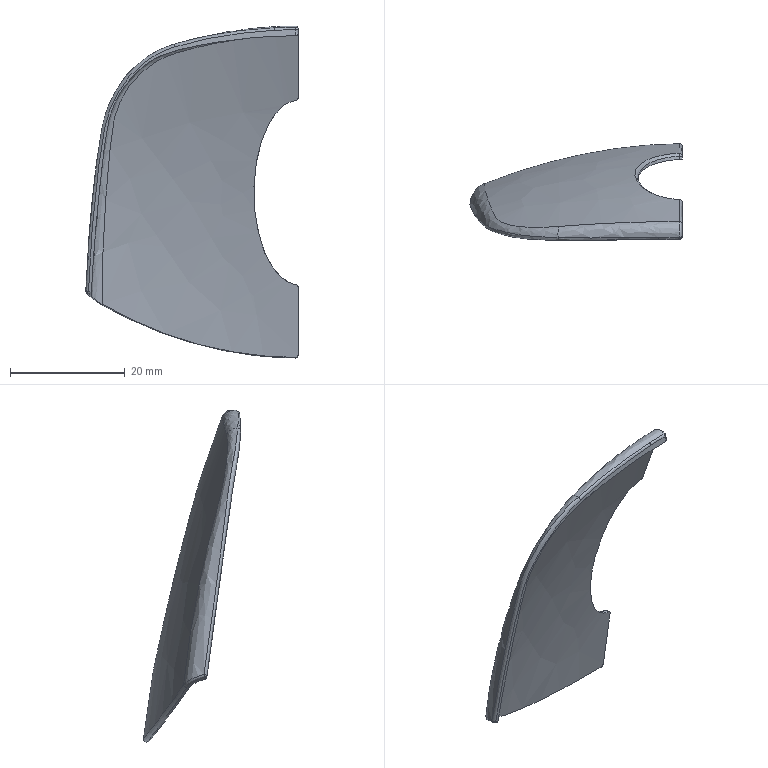Part | STEP file | Guide wheel mechanism revised.sldasm-Part-308 | 1 solid | 33 faces | box 37.055 x 16.939 x 57.91 mm | volume 1764 mm3 | spline 27 | cylinder 4 | plane 2 | commonest cylinder face diameters 1 x4